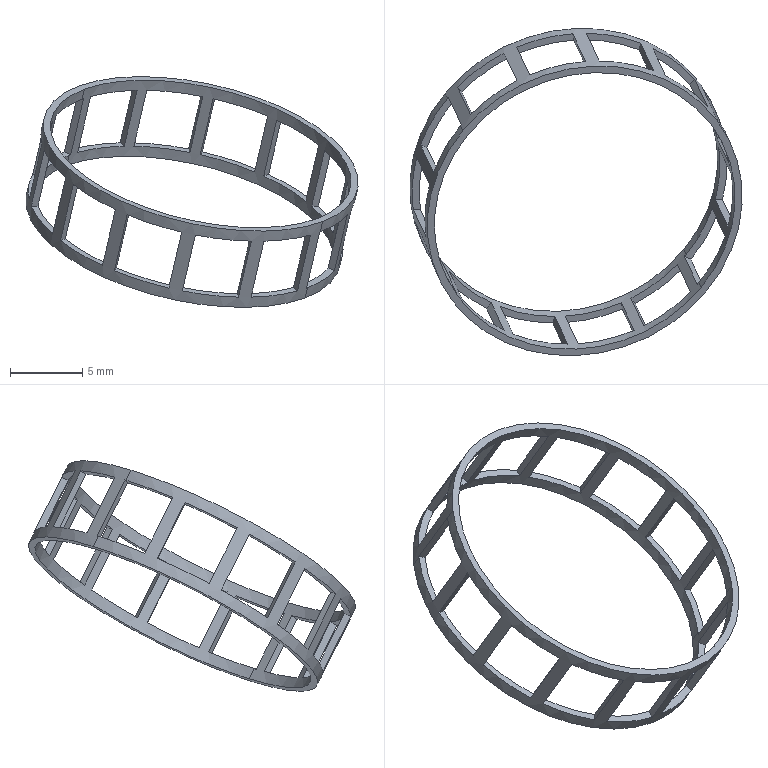Part | SolidWorks | features BaseBody 1 | 1 solid | 62 faces | box 22.954 x 22.595 x 15.926 mm | volume 80.609 mm3 | plane 58 | cylinder 4 | commonest cylinder face diameters 21.2 x2 22.2 x2